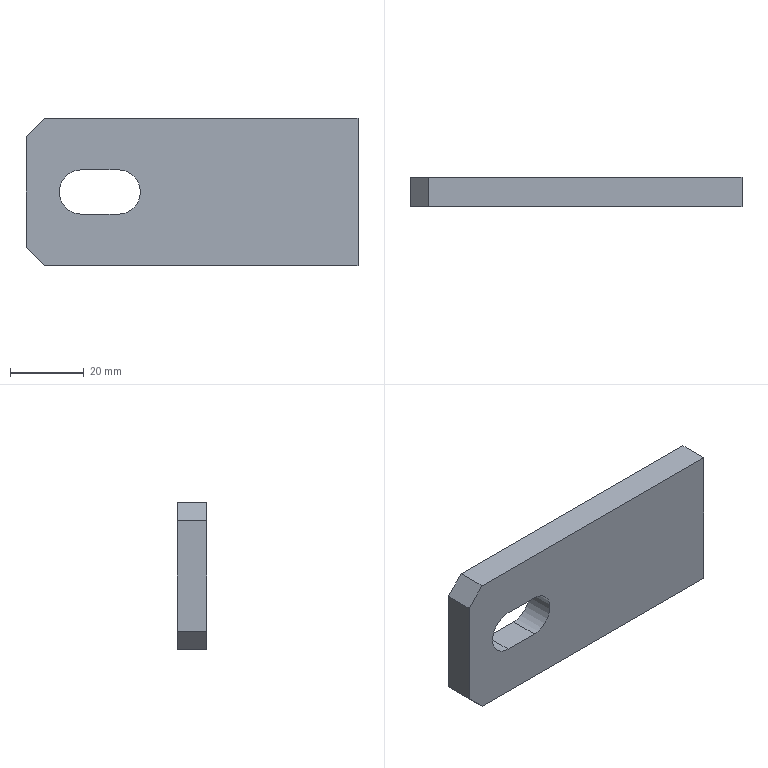Part | STEP file | E3-Guardrail base plate 1 | 1 solid | 12 faces | box 90 x 8 x 40 mm | volume 26735 mm3 | plane 10 | cylinder 2 | commonest cylinder face diameters 12 x2
STEP:
#1=CARTESIAN_POINT('',(0.,0.,0.));
#2=DIRECTION('',(0.,0.,1.));
#3=DIRECTION('',(1.,0.,0.));
#4=AXIS2_PLACEMENT_3D('',#1,#2,#3);
#5=CARTESIAN_POINT('',(45.,0.,-20.));
#6=VERTEX_POINT('',#5);
#7=CARTESIAN_POINT('',(45.,0.,20.));
#8=VERTEX_POINT('',#7);
#9=CARTESIAN_POINT('',(45.,0.,20.));
#10=DIRECTION('',(0.,0.,1.));
#11=VECTOR('',#10,1.);
#12=LINE('',#9,#11);
#13=CARTESIAN_POINT('',(45.,8.,20.));
#14=DIRECTION('',(-1.,0.,0.));
#15=DIRECTION('',(0.,0.,-1.));
#16=AXIS2_PLACEMENT_3D('',#13,#14,#15);
#17=PLANE('',#16);
#18=CARTESIAN_POINT('',(0.,8.));
#19=DIRECTION('',(-1.,0.));
#20=VECTOR('',#19,1.);
#21=LINE('',#18,#20);
#22=(GEOMETRIC_REPRESENTATION_CONTEXT(2)PARAMETRIC_REPRESENTATION_CONTEXT()REPRESENTATION_CONTEXT('',''));
#23=DEFINITIONAL_REPRESENTATION('',(#21),#22);
#24=PCURVE('',#17,#23);
#25=CARTESIAN_POINT('',(0.,0.,0.));
#26=DIRECTION('',(0.,1.,0.));
#27=DIRECTION('',(0.,0.,-1.));
#28=AXIS2_PLACEMENT_3D('',#25,#26,#27);
#29=PLANE('',#28);
#30=CARTESIAN_POINT('',(-20.,-45.));
#31=DIRECTION('',(-1.,0.));
#32=VECTOR('',#31,1.);
#33=LINE('',#30,#32);
#34=(GEOMETRIC_REPRESENTATION_CONTEXT(2)PARAMETRIC_REPRESENTATION_CONTEXT()REPRESENTATION_CONTEXT('',''));
#35=DEFINITIONAL_REPRESENTATION('',(#33),#34);
#36=PCURVE('',#29,#35);
#37=SURFACE_CURVE('',#12,(#24,#36),.PCURVE_S1.);
#38=EDGE_CURVE('',#6,#8,#37,.T.);
#39=ORIENTED_EDGE('',*,*,#38,.F.);
#40=CARTESIAN_POINT('',(45.,8.,-20.));
#41=VERTEX_POINT('',#40);
#42=CARTESIAN_POINT('',(45.,8.,-20.));
#43=DIRECTION('',(0.,-1.,0.));
#44=VECTOR('',#43,1.);
#45=LINE('',#42,#44);
#46=CARTESIAN_POINT('',(40.,0.));
#47=DIRECTION('',(0.,1.));
#48=VECTOR('',#47,1.);
#49=LINE('',#46,#48);
#50=(GEOMETRIC_REPRESENTATION_CONTEXT(2)PARAMETRIC_REPRESENTATION_CONTEXT()REPRESENTATION_CONTEXT('',''));
#51=DEFINITIONAL_REPRESENTATION('',(#49),#50);
#52=PCURVE('',#17,#51);
#53=CARTESIAN_POINT('',(-45.,8.,-20.));
#54=DIRECTION('',(0.,0.,1.));
#55=DIRECTION('',(-1.,0.,0.));
#56=AXIS2_PLACEMENT_3D('',#53,#54,#55);
#57=PLANE('',#56);
#58=CARTESIAN_POINT('',(-90.,0.));
#59=DIRECTION('',(0.,1.));
#60=VECTOR('',#59,1.);
#61=LINE('',#58,#60);
#62=(GEOMETRIC_REPRESENTATION_CONTEXT(2)PARAMETRIC_REPRESENTATION_CONTEXT()REPRESENTATION_CONTEXT('',''));
#63=DEFINITIONAL_REPRESENTATION('',(#61),#62);
#64=PCURVE('',#57,#63);
#65=SURFACE_CURVE('',#45,(#52,#64),.PCURVE_S1.);
#66=EDGE_CURVE('',#41,#6,#65,.T.);
#67=ORIENTED_EDGE('',*,*,#66,.F.);
#68=CARTESIAN_POINT('',(45.,8.,20.));
#69=VERTEX_POINT('',#68);
#70=CARTESIAN_POINT('',(45.,8.,20.));
#71=DIRECTION('',(0.,0.,1.));
#72=VECTOR('',#71,1.);
#73=LINE('',#70,#72);
#74=CARTESIAN_POINT('',(0.,0.));
#75=DIRECTION('',(-1.,0.));
#76=VECTOR('',#75,1.);
#77=LINE('',#74,#76);
#78=(GEOMETRIC_REPRESENTATION_CONTEXT(2)PARAMETRIC_REPRESENTATION_CONTEXT()REPRESENTATION_CONTEXT('',''));
#79=DEFINITIONAL_REPRESENTATION('',(#77),#78);
#80=PCURVE('',#17,#79);
#81=CARTESIAN_POINT('',(0.,8.,0.));
#82=DIRECTION('',(0.,1.,0.));
#83=DIRECTION('',(0.,0.,-1.));
#84=AXIS2_PLACEMENT_3D('',#81,#82,#83);
#85=PLANE('',#84);
#86=CARTESIAN_POINT('',(-20.,-45.));
#87=DIRECTION('',(-1.,0.));
#88=VECTOR('',#87,1.);
#89=LINE('',#86,#88);
#90=(GEOMETRIC_REPRESENTATION_CONTEXT(2)PARAMETRIC_REPRESENTATION_CONTEXT()REPRESENTATION_CONTEXT('',''));
#91=DEFINITIONAL_REPRESENTATION('',(#89),#90);
#92=PCURVE('',#85,#91);
#93=SURFACE_CURVE('',#73,(#80,#92),.PCURVE_S1.);
#94=EDGE_CURVE('',#41,#69,#93,.T.);
#95=ORIENTED_EDGE('',*,*,#94,.T.);
#96=CARTESIAN_POINT('',(45.,8.,20.));
#97=DIRECTION('',(0.,-1.,0.));
#98=VECTOR('',#97,1.);
#99=LINE('',#96,#98);
#100=CARTESIAN_POINT('',(0.,0.));
#101=DIRECTION('',(0.,1.));
#102=VECTOR('',#101,1.);
#103=LINE('',#100,#102);
#104=(GEOMETRIC_REPRESENTATION_CONTEXT(2)PARAMETRIC_REPRESENTATION_CONTEXT()REPRESENTATION_CONTEXT('',''));
#105=DEFINITIONAL_REPRESENTATION('',(#103),#104);
#106=PCURVE('',#17,#105);
#107=CARTESIAN_POINT('',(-45.,8.,20.));
#108=DIRECTION('',(0.,0.,-1.));
#109=DIRECTION('',(1.,0.,0.));
#110=AXIS2_PLACEMENT_3D('',#107,#108,#109);
#111=PLANE('',#110);
#112=CARTESIAN_POINT('',(90.,0.));
#113=DIRECTION('',(0.,1.));
#114=VECTOR('',#113,1.);
#115=LINE('',#112,#114);
#116=(GEOMETRIC_REPRESENTATION_CONTEXT(2)PARAMETRIC_REPRESENTATION_CONTEXT()REPRESENTATION_CONTEXT('',''));
#117=DEFINITIONAL_REPRESENTATION('',(#115),#116);
#118=PCURVE('',#111,#117);
#119=SURFACE_CURVE('',#99,(#106,#118),.PCURVE_S1.);
#120=EDGE_CURVE('',#69,#8,#119,.T.);
#121=ORIENTED_EDGE('',*,*,#120,.T.);
#122=EDGE_LOOP('',(#39,#67,#95,#121));
#123=FACE_BOUND('',#122,.T.);
#124=ADVANCED_FACE('',(#123),#17,.F.);
#125=CARTESIAN_POINT('',(-40.,0.,20.));
#126=VERTEX_POINT('',#125);
#127=CARTESIAN_POINT('',(-45.,0.,20.));
#128=DIRECTION('',(-1.,0.,0.));
#129=VECTOR('',#128,1.);
#130=LINE('',#127,#129);
#131=CARTESIAN_POINT('',(0.,8.));
#132=DIRECTION('',(-1.,0.));
#133=VECTOR('',#132,1.);
#134=LINE('',#131,#133);
#135=(GEOMETRIC_REPRESENTATION_CONTEXT(2)PARAMETRIC_REPRESENTATION_CONTEXT()REPRESENTATION_CONTEXT('',''));
#136=DEFINITIONAL_REPRESENTATION('',(#134),#135);
#137=PCURVE('',#111,#136);
#138=CARTESIAN_POINT('',(-20.,45.));
#139=DIRECTION('',(0.,1.));
#140=VECTOR('',#139,1.);
#141=LINE('',#138,#140);
#142=(GEOMETRIC_REPRESENTATION_CONTEXT(2)PARAMETRIC_REPRESENTATION_CONTEXT()REPRESENTATION_CONTEXT('',''));
#143=DEFINITIONAL_REPRESENTATION('',(#141),#142);
#144=PCURVE('',#29,#143);
#145=SURFACE_CURVE('',#130,(#137,#144),.PCURVE_S1.);
#146=EDGE_CURVE('',#8,#126,#145,.T.);
#147=ORIENTED_EDGE('',*,*,#146,.F.);
#148=ORIENTED_EDGE('',*,*,#120,.F.);
#149=CARTESIAN_POINT('',(-40.,8.,20.));
#150=VERTEX_POINT('',#149);
#151=CARTESIAN_POINT('',(-45.,8.,20.));
#152=DIRECTION('',(-1.,0.,0.));
#153=VECTOR('',#152,1.);
#154=LINE('',#151,#153);
#155=CARTESIAN_POINT('',(0.,0.));
#156=DIRECTION('',(-1.,0.));
#157=VECTOR('',#156,1.);
#158=LINE('',#155,#157);
#159=(GEOMETRIC_REPRESENTATION_CONTEXT(2)PARAMETRIC_REPRESENTATION_CONTEXT()REPRESENTATION_CONTEXT('',''));
#160=DEFINITIONAL_REPRESENTATION('',(#158),#159);
#161=PCURVE('',#111,#160);
#162=CARTESIAN_POINT('',(-20.,45.));
#163=DIRECTION('',(0.,1.));
#164=VECTOR('',#163,1.);
#165=LINE('',#162,#164);
#166=(GEOMETRIC_REPRESENTATION_CONTEXT(2)PARAMETRIC_REPRESENTATION_CONTEXT()REPRESENTATION_CONTEXT('',''));
#167=DEFINITIONAL_REPRESENTATION('',(#165),#166);
#168=PCURVE('',#85,#167);
#169=SURFACE_CURVE('',#154,(#161,#168),.PCURVE_S1.);
#170=EDGE_CURVE('',#69,#150,#169,.T.);
#171=ORIENTED_EDGE('',*,*,#170,.T.);
#172=CARTESIAN_POINT('',(-40.,8.,20.));
#173=DIRECTION('',(0.,1.,0.));
#174=VECTOR('',#173,1.);
#175=LINE('',#172,#174);
#176=CARTESIAN_POINT('',(5.,0.));
#177=DIRECTION('',(0.,-1.));
#178=VECTOR('',#177,1.);
#179=LINE('',#176,#178);
#180=(GEOMETRIC_REPRESENTATION_CONTEXT(2)PARAMETRIC_REPRESENTATION_CONTEXT()REPRESENTATION_CONTEXT('',''));
#181=DEFINITIONAL_REPRESENTATION('',(#179),#180);
#182=PCURVE('',#111,#181);
#183=CARTESIAN_POINT('',(-45.,8.,15.));
#184=DIRECTION('',(0.7071,0.,-0.7071));
#185=DIRECTION('',(0.,-1.,0.));
#186=AXIS2_PLACEMENT_3D('',#183,#184,#185);
#187=PLANE('',#186);
#188=CARTESIAN_POINT('',(0.,-7.071));
#189=DIRECTION('',(-1.,0.));
#190=VECTOR('',#189,1.);
#191=LINE('',#188,#190);
#192=(GEOMETRIC_REPRESENTATION_CONTEXT(2)PARAMETRIC_REPRESENTATION_CONTEXT()REPRESENTATION_CONTEXT('',''));
#193=DEFINITIONAL_REPRESENTATION('',(#191),#192);
#194=PCURVE('',#187,#193);
#195=SURFACE_CURVE('',#175,(#182,#194),.PCURVE_S1.);
#196=EDGE_CURVE('',#126,#150,#195,.T.);
#197=ORIENTED_EDGE('',*,*,#196,.F.);
#198=EDGE_LOOP('',(#147,#148,#171,#197));
#199=FACE_BOUND('',#198,.T.);
#200=ADVANCED_FACE('',(#199),#111,.F.);
#201=CARTESIAN_POINT('',(-45.,0.,15.));
#202=VERTEX_POINT('',#201);
#203=CARTESIAN_POINT('',(-45.,0.,-15.));
#204=VERTEX_POINT('',#203);
#205=CARTESIAN_POINT('',(-45.,0.,20.));
#206=DIRECTION('',(0.,0.,-1.));
#207=VECTOR('',#206,1.);
#208=LINE('',#205,#207);
#209=CARTESIAN_POINT('',(-45.,8.,20.));
#210=DIRECTION('',(1.,0.,0.));
#211=DIRECTION('',(0.,0.,1.));
#212=AXIS2_PLACEMENT_3D('',#209,#210,#211);
#213=PLANE('',#212);
#214=CARTESIAN_POINT('',(0.,8.));
#215=DIRECTION('',(-1.,0.));
#216=VECTOR('',#215,1.);
#217=LINE('',#214,#216);
#218=(GEOMETRIC_REPRESENTATION_CONTEXT(2)PARAMETRIC_REPRESENTATION_CONTEXT()REPRESENTATION_CONTEXT('',''));
#219=DEFINITIONAL_REPRESENTATION('',(#217),#218);
#220=PCURVE('',#213,#219);
#221=CARTESIAN_POINT('',(-20.,45.));
#222=DIRECTION('',(1.,0.));
#223=VECTOR('',#222,1.);
#224=LINE('',#221,#223);
#225=(GEOMETRIC_REPRESENTATION_CONTEXT(2)PARAMETRIC_REPRESENTATION_CONTEXT()REPRESENTATION_CONTEXT('',''));
#226=DEFINITIONAL_REPRESENTATION('',(#224),#225);
#227=PCURVE('',#29,#226);
#228=SURFACE_CURVE('',#208,(#220,#227),.PCURVE_S1.);
#229=EDGE_CURVE('',#202,#204,#228,.T.);
#230=ORIENTED_EDGE('',*,*,#229,.F.);
#231=CARTESIAN_POINT('',(-45.,8.,15.));
#232=VERTEX_POINT('',#231);
#233=CARTESIAN_POINT('',(-45.,8.,15.));
#234=DIRECTION('',(0.,-1.,0.));
#235=VECTOR('',#234,1.);
#236=LINE('',#233,#235);
#237=CARTESIAN_POINT('',(-5.,0.));
#238=DIRECTION('',(0.,1.));
#239=VECTOR('',#238,1.);
#240=LINE('',#237,#239);
#241=(GEOMETRIC_REPRESENTATION_CONTEXT(2)PARAMETRIC_REPRESENTATION_CONTEXT()REPRESENTATION_CONTEXT('',''));
#242=DEFINITIONAL_REPRESENTATION('',(#240),#241);
#243=PCURVE('',#213,#242);
#244=CARTESIAN_POINT('',(0.,0.));
#245=DIRECTION('',(1.,0.));
#246=VECTOR('',#245,1.);
#247=LINE('',#244,#246);
#248=(GEOMETRIC_REPRESENTATION_CONTEXT(2)PARAMETRIC_REPRESENTATION_CONTEXT()REPRESENTATION_CONTEXT('',''));
#249=DEFINITIONAL_REPRESENTATION('',(#247),#248);
#250=PCURVE('',#187,#249);
#251=SURFACE_CURVE('',#236,(#243,#250),.PCURVE_S1.);
#252=EDGE_CURVE('',#232,#202,#251,.T.);
#253=ORIENTED_EDGE('',*,*,#252,.F.);
#254=CARTESIAN_POINT('',(-45.,8.,-15.));
#255=VERTEX_POINT('',#254);
#256=CARTESIAN_POINT('',(-45.,8.,20.));
#257=DIRECTION('',(0.,0.,-1.));
#258=VECTOR('',#257,1.);
#259=LINE('',#256,#258);
#260=CARTESIAN_POINT('',(0.,0.));
#261=DIRECTION('',(-1.,0.));
#262=VECTOR('',#261,1.);
#263=LINE('',#260,#262);
#264=(GEOMETRIC_REPRESENTATION_CONTEXT(2)PARAMETRIC_REPRESENTATION_CONTEXT()REPRESENTATION_CONTEXT('',''));
#265=DEFINITIONAL_REPRESENTATION('',(#263),#264);
#266=PCURVE('',#213,#265);
#267=CARTESIAN_POINT('',(-20.,45.));
#268=DIRECTION('',(1.,0.));
#269=VECTOR('',#268,1.);
#270=LINE('',#267,#269);
#271=(GEOMETRIC_REPRESENTATION_CONTEXT(2)PARAMETRIC_REPRESENTATION_CONTEXT()REPRESENTATION_CONTEXT('',''));
#272=DEFINITIONAL_REPRESENTATION('',(#270),#271);
#273=PCURVE('',#85,#272);
#274=SURFACE_CURVE('',#259,(#266,#273),.PCURVE_S1.);
#275=EDGE_CURVE('',#232,#255,#274,.T.);
#276=ORIENTED_EDGE('',*,*,#275,.T.);
#277=CARTESIAN_POINT('',(-45.,8.,-15.));
#278=DIRECTION('',(0.,1.,0.));
#279=VECTOR('',#278,1.);
#280=LINE('',#277,#279);
#281=CARTESIAN_POINT('',(-35.,0.));
#282=DIRECTION('',(0.,-1.));
#283=VECTOR('',#282,1.);
#284=LINE('',#281,#283);
#285=(GEOMETRIC_REPRESENTATION_CONTEXT(2)PARAMETRIC_REPRESENTATION_CONTEXT()REPRESENTATION_CONTEXT('',''));
#286=DEFINITIONAL_REPRESENTATION('',(#284),#285);
#287=PCURVE('',#213,#286);
#288=CARTESIAN_POINT('',(-40.,8.,-20.));
#289=DIRECTION('',(0.7071,0.,0.7071));
#290=DIRECTION('',(0.,-1.,0.));
#291=AXIS2_PLACEMENT_3D('',#288,#289,#290);
#292=PLANE('',#291);
#293=CARTESIAN_POINT('',(0.,-7.071));
#294=DIRECTION('',(-1.,0.));
#295=VECTOR('',#294,1.);
#296=LINE('',#293,#295);
#297=(GEOMETRIC_REPRESENTATION_CONTEXT(2)PARAMETRIC_REPRESENTATION_CONTEXT()REPRESENTATION_CONTEXT('',''));
#298=DEFINITIONAL_REPRESENTATION('',(#296),#297);
#299=PCURVE('',#292,#298);
#300=SURFACE_CURVE('',#280,(#287,#299),.PCURVE_S1.);
#301=EDGE_CURVE('',#204,#255,#300,.T.);
#302=ORIENTED_EDGE('',*,*,#301,.F.);
#303=EDGE_LOOP('',(#230,#253,#276,#302));
#304=FACE_BOUND('',#303,.T.);
#305=ADVANCED_FACE('',(#304),#213,.F.);
#306=CARTESIAN_POINT('',(-40.,8.,-20.));
#307=VERTEX_POINT('',#306);
#308=CARTESIAN_POINT('',(-45.,8.,-20.));
#309=DIRECTION('',(1.,0.,0.));
#310=VECTOR('',#309,1.);
#311=LINE('',#308,#310);
#312=CARTESIAN_POINT('',(0.,0.));
#313=DIRECTION('',(-1.,0.));
#314=VECTOR('',#313,1.);
#315=LINE('',#312,#314);
#316=(GEOMETRIC_REPRESENTATION_CONTEXT(2)PARAMETRIC_REPRESENTATION_CONTEXT()REPRESENTATION_CONTEXT('',''));
#317=DEFINITIONAL_REPRESENTATION('',(#315),#316);
#318=PCURVE('',#57,#317);
#319=CARTESIAN_POINT('',(20.,45.));
#320=DIRECTION('',(0.,-1.));
#321=VECTOR('',#320,1.);
#322=LINE('',#319,#321);
#323=(GEOMETRIC_REPRESENTATION_CONTEXT(2)PARAMETRIC_REPRESENTATION_CONTEXT()REPRESENTATION_CONTEXT('',''));
#324=DEFINITIONAL_REPRESENTATION('',(#322),#323);
#325=PCURVE('',#85,#324);
#326=SURFACE_CURVE('',#311,(#318,#325),.PCURVE_S1.);
#327=EDGE_CURVE('',#307,#41,#326,.T.);
#328=ORIENTED_EDGE('',*,*,#327,.T.);
#329=ORIENTED_EDGE('',*,*,#66,.T.);
#330=CARTESIAN_POINT('',(-40.,0.,-20.));
#331=VERTEX_POINT('',#330);
#332=CARTESIAN_POINT('',(-45.,0.,-20.));
#333=DIRECTION('',(1.,0.,0.));
#334=VECTOR('',#333,1.);
#335=LINE('',#332,#334);
#336=CARTESIAN_POINT('',(0.,8.));
#337=DIRECTION('',(-1.,0.));
#338=VECTOR('',#337,1.);
#339=LINE('',#336,#338);
#340=(GEOMETRIC_REPRESENTATION_CONTEXT(2)PARAMETRIC_REPRESENTATION_CONTEXT()REPRESENTATION_CONTEXT('',''));
#341=DEFINITIONAL_REPRESENTATION('',(#339),#340);
#342=PCURVE('',#57,#341);
#343=CARTESIAN_POINT('',(20.,45.));
#344=DIRECTION('',(0.,-1.));
#345=VECTOR('',#344,1.);
#346=LINE('',#343,#345);
#347=(GEOMETRIC_REPRESENTATION_CONTEXT(2)PARAMETRIC_REPRESENTATION_CONTEXT()REPRESENTATION_CONTEXT('',''));
#348=DEFINITIONAL_REPRESENTATION('',(#346),#347);
#349=PCURVE('',#29,#348);
#350=SURFACE_CURVE('',#335,(#342,#349),.PCURVE_S1.);
#351=EDGE_CURVE('',#331,#6,#350,.T.);
#352=ORIENTED_EDGE('',*,*,#351,.F.);
#353=CARTESIAN_POINT('',(-40.,8.,-20.));
#354=DIRECTION('',(0.,-1.,0.));
#355=VECTOR('',#354,1.);
#356=LINE('',#353,#355);
#357=CARTESIAN_POINT('',(-5.,0.));
#358=DIRECTION('',(0.,1.));
#359=VECTOR('',#358,1.);
#360=LINE('',#357,#359);
#361=(GEOMETRIC_REPRESENTATION_CONTEXT(2)PARAMETRIC_REPRESENTATION_CONTEXT()REPRESENTATION_CONTEXT('',''));
#362=DEFINITIONAL_REPRESENTATION('',(#360),#361);
#363=PCURVE('',#57,#362);
#364=CARTESIAN_POINT('',(0.,0.));
#365=DIRECTION('',(1.,0.));
#366=VECTOR('',#365,1.);
#367=LINE('',#364,#366);
#368=(GEOMETRIC_REPRESENTATION_CONTEXT(2)PARAMETRIC_REPRESENTATION_CONTEXT()REPRESENTATION_CONTEXT('',''));
#369=DEFINITIONAL_REPRESENTATION('',(#367),#368);
#370=PCURVE('',#292,#369);
#371=SURFACE_CURVE('',#356,(#363,#370),.PCURVE_S1.);
#372=EDGE_CURVE('',#307,#331,#371,.T.);
#373=ORIENTED_EDGE('',*,*,#372,.F.);
#374=EDGE_LOOP('',(#328,#329,#352,#373));
#375=FACE_BOUND('',#374,.T.);
#376=ADVANCED_FACE('',(#375),#57,.F.);
#377=CARTESIAN_POINT('',(-20.,8.,-6.));
#378=VERTEX_POINT('',#377);
#379=CARTESIAN_POINT('',(-20.,8.,6.));
#380=VERTEX_POINT('',#379);
#381=CARTESIAN_POINT('',(-20.,8.,0.));
#382=DIRECTION('',(0.,-1.,0.));
#383=DIRECTION('',(0.,0.,-1.));
#384=AXIS2_PLACEMENT_3D('',#381,#382,#383);
#385=CIRCLE('',#384,6.);
#386=CARTESIAN_POINT('',(6.,20.));
#387=CARTESIAN_POINT('',(6.,9.608));
#388=CARTESIAN_POINT('',(-3.,14.804));
#389=CARTESIAN_POINT('',(-12.,20.));
#390=CARTESIAN_POINT('',(-3.,25.196));
#391=CARTESIAN_POINT('',(6.,30.392));
#392=CARTESIAN_POINT('',(6.,20.));
#393=(BOUNDED_CURVE()B_SPLINE_CURVE(2,(#386,#387,#388,#389,#390,#391,#392),.UNSPECIFIED.,.T.,.F.)B_SPLINE_CURVE_WITH_KNOTS((1,2,2,2,2,1),(-2.094,0.,2.094,4.189,6.283,8.378),.UNSPECIFIED.)CURVE()GEOMETRIC_REPRESENTATION_ITEM()RATIONAL_B_SPLINE_CURVE((1.,0.5,1.,0.5,1.,0.5,1.))REPRESENTATION_ITEM(''));
#394=(GEOMETRIC_REPRESENTATION_CONTEXT(2)PARAMETRIC_REPRESENTATION_CONTEXT()REPRESENTATION_CONTEXT('',''));
#395=DEFINITIONAL_REPRESENTATION('',(#393),#394);
#396=PCURVE('',#85,#395);
#397=CARTESIAN_POINT('',(-20.,8.,0.));
#398=DIRECTION('',(0.,1.,0.));
#399=DIRECTION('',(0.,0.,-1.));
#400=AXIS2_PLACEMENT_3D('',#397,#398,#399);
#401=CYLINDRICAL_SURFACE('',#400,6.);
#402=CARTESIAN_POINT('',(6.283,0.));
#403=DIRECTION('',(-1.,0.));
#404=VECTOR('',#403,1.);
#405=LINE('',#402,#404);
#406=(GEOMETRIC_REPRESENTATION_CONTEXT(2)PARAMETRIC_REPRESENTATION_CONTEXT()REPRESENTATION_CONTEXT('',''));
#407=DEFINITIONAL_REPRESENTATION('',(#405),#406);
#408=PCURVE('',#401,#407);
#409=SURFACE_CURVE('',#385,(#396,#408),.PCURVE_S1.);
#410=EDGE_CURVE('',#378,#380,#409,.T.);
#411=ORIENTED_EDGE('',*,*,#410,.T.);
#412=CARTESIAN_POINT('',(-30.,8.,6.));
#413=VERTEX_POINT('',#412);
#414=CARTESIAN_POINT('',(-30.,8.,6.));
#415=DIRECTION('',(1.,0.,0.));
#416=VECTOR('',#415,1.);
#417=LINE('',#414,#416);
#418=CARTESIAN_POINT('',(-6.,30.));
#419=DIRECTION('',(0.,-1.));
#420=VECTOR('',#419,1.);
#421=LINE('',#418,#420);
#422=(GEOMETRIC_REPRESENTATION_CONTEXT(2)PARAMETRIC_REPRESENTATION_CONTEXT()REPRESENTATION_CONTEXT('',''));
#423=DEFINITIONAL_REPRESENTATION('',(#421),#422);
#424=PCURVE('',#85,#423);
#425=CARTESIAN_POINT('',(-30.,8.,6.));
#426=DIRECTION('',(0.,0.,1.));
#427=DIRECTION('',(-1.,0.,0.));
#428=AXIS2_PLACEMENT_3D('',#425,#426,#427);
#429=PLANE('',#428);
#430=CARTESIAN_POINT('',(0.,0.));
#431=DIRECTION('',(-1.,0.));
#432=VECTOR('',#431,1.);
#433=LINE('',#430,#432);
#434=(GEOMETRIC_REPRESENTATION_CONTEXT(2)PARAMETRIC_REPRESENTATION_CONTEXT()REPRESENTATION_CONTEXT('',''));
#435=DEFINITIONAL_REPRESENTATION('',(#433),#434);
#436=PCURVE('',#429,#435);
#437=SURFACE_CURVE('',#417,(#424,#436),.PCURVE_S1.);
#438=EDGE_CURVE('',#413,#380,#437,.T.);
#439=ORIENTED_EDGE('',*,*,#438,.F.);
#440=CARTESIAN_POINT('',(-30.,8.,-6.));
#441=VERTEX_POINT('',#440);
#442=CARTESIAN_POINT('',(-30.,8.,0.));
#443=DIRECTION('',(0.,-1.,0.));
#444=DIRECTION('',(0.,0.,-1.));
#445=AXIS2_PLACEMENT_3D('',#442,#443,#444);
#446=CIRCLE('',#445,6.);
#447=CARTESIAN_POINT('',(6.,30.));
#448=CARTESIAN_POINT('',(6.,19.608));
#449=CARTESIAN_POINT('',(-3.,24.804));
#450=CARTESIAN_POINT('',(-12.,30.));
#451=CARTESIAN_POINT('',(-3.,35.196));
#452=CARTESIAN_POINT('',(6.,40.392));
#453=CARTESIAN_POINT('',(6.,30.));
#454=(BOUNDED_CURVE()B_SPLINE_CURVE(2,(#447,#448,#449,#450,#451,#452,#453),.UNSPECIFIED.,.T.,.F.)B_SPLINE_CURVE_WITH_KNOTS((1,2,2,2,2,1),(-2.094,0.,2.094,4.189,6.283,8.378),.UNSPECIFIED.)CURVE()GEOMETRIC_REPRESENTATION_ITEM()RATIONAL_B_SPLINE_CURVE((1.,0.5,1.,0.5,1.,0.5,1.))REPRESENTATION_ITEM(''));
#455=(GEOMETRIC_REPRESENTATION_CONTEXT(2)PARAMETRIC_REPRESENTATION_CONTEXT()REPRESENTATION_CONTEXT('',''));
#456=DEFINITIONAL_REPRESENTATION('',(#454),#455);
#457=PCURVE('',#85,#456);
#458=CARTESIAN_POINT('',(-30.,8.,0.));
#459=DIRECTION('',(0.,1.,0.));
#460=DIRECTION('',(0.,0.,-1.));
#461=AXIS2_PLACEMENT_3D('',#458,#459,#460);
#462=CYLINDRICAL_SURFACE('',#461,6.);
#463=CARTESIAN_POINT('',(6.283,0.));
#464=DIRECTION('',(-1.,0.));
#465=VECTOR('',#464,1.);
#466=LINE('',#463,#465);
#467=(GEOMETRIC_REPRESENTATION_CONTEXT(2)PARAMETRIC_REPRESENTATION_CONTEXT()REPRESENTATION_CONTEXT('',''));
#468=DEFINITIONAL_REPRESENTATION('',(#466),#467);
#469=PCURVE('',#462,#468);
#470=SURFACE_CURVE('',#446,(#457,#469),.PCURVE_S1.);
#471=EDGE_CURVE('',#413,#441,#470,.T.);
#472=ORIENTED_EDGE('',*,*,#471,.T.);
#473=CARTESIAN_POINT('',(-30.,8.,-6.));
#474=DIRECTION('',(1.,0.,0.));
#475=VECTOR('',#474,1.);
#476=LINE('',#473,#475);
#477=CARTESIAN_POINT('',(6.,30.));
#478=DIRECTION('',(0.,-1.));
#479=VECTOR('',#478,1.);
#480=LINE('',#477,#479);
#481=(GEOMETRIC_REPRESENTATION_CONTEXT(2)PARAMETRIC_REPRESENTATION_CONTEXT()REPRESENTATION_CONTEXT('',''));
#482=DEFINITIONAL_REPRESENTATION('',(#480),#481);
#483=PCURVE('',#85,#482);
#484=CARTESIAN_POINT('',(-30.,8.,-6.));
#485=DIRECTION('',(0.,0.,-1.));
#486=DIRECTION('',(1.,0.,0.));
#487=AXIS2_PLACEMENT_3D('',#484,#485,#486);
#488=PLANE('',#487);
#489=CARTESIAN_POINT('',(0.,0.));
#490=DIRECTION('',(1.,0.));
#491=VECTOR('',#490,1.);
#492=LINE('',#489,#491);
#493=(GEOMETRIC_REPRESENTATION_CONTEXT(2)PARAMETRIC_REPRESENTATION_CONTEXT()REPRESENTATION_CONTEXT('',''));
#494=DEFINITIONAL_REPRESENTATION('',(#492),#493);
#495=PCURVE('',#488,#494);
#496=SURFACE_CURVE('',#476,(#483,#495),.PCURVE_S1.);
#497=EDGE_CURVE('',#441,#378,#496,.T.);
#498=ORIENTED_EDGE('',*,*,#497,.T.);
#499=EDGE_LOOP('',(#411,#439,#472,#498));
#500=FACE_BOUND('',#499,.T.);
#501=ORIENTED_EDGE('',*,*,#275,.F.);
#502=CARTESIAN_POINT('',(-30.,8.,30.));
#503=DIRECTION('',(-0.7071,0.,-0.7071));
#504=VECTOR('',#503,1.);
#505=LINE('',#502,#504);
#506=CARTESIAN_POINT('',(-30.,30.));
#507=DIRECTION('',(0.7071,0.7071));
#508=VECTOR('',#507,1.);
#509=LINE('',#506,#508);
#510=(GEOMETRIC_REPRESENTATION_CONTEXT(2)PARAMETRIC_REPRESENTATION_CONTEXT()REPRESENTATION_CONTEXT('',''));
#511=DEFINITIONAL_REPRESENTATION('',(#509),#510);
#512=PCURVE('',#85,#511);
#513=CARTESIAN_POINT('',(0.,-21.213));
#514=DIRECTION('',(0.,1.));
#515=VECTOR('',#514,1.);
#516=LINE('',#513,#515);
#517=(GEOMETRIC_REPRESENTATION_CONTEXT(2)PARAMETRIC_REPRESENTATION_CONTEXT()REPRESENTATION_CONTEXT('',''));
#518=DEFINITIONAL_REPRESENTATION('',(#516),#517);
#519=PCURVE('',#187,#518);
#520=SURFACE_CURVE('',#505,(#512,#519),.PCURVE_S1.);
#521=EDGE_CURVE('',#150,#232,#520,.T.);
#522=ORIENTED_EDGE('',*,*,#521,.F.);
#523=ORIENTED_EDGE('',*,*,#170,.F.);
#524=ORIENTED_EDGE('',*,*,#94,.F.);
#525=ORIENTED_EDGE('',*,*,#327,.F.);
#526=CARTESIAN_POINT('',(-30.,8.,-30.));
#527=DIRECTION('',(0.7071,0.,-0.7071));
#528=VECTOR('',#527,1.);
#529=LINE('',#526,#528);
#530=CARTESIAN_POINT('',(30.,30.));
#531=DIRECTION('',(0.7071,-0.7071));
#532=VECTOR('',#531,1.);
#533=LINE('',#530,#532);
#534=(GEOMETRIC_REPRESENTATION_CONTEXT(2)PARAMETRIC_REPRESENTATION_CONTEXT()REPRESENTATION_CONTEXT('',''));
#535=DEFINITIONAL_REPRESENTATION('',(#533),#534);
#536=PCURVE('',#85,#535);
#537=CARTESIAN_POINT('',(0.,14.142));
#538=DIRECTION('',(0.,1.));
#539=VECTOR('',#538,1.);
#540=LINE('',#537,#539);
#541=(GEOMETRIC_REPRESENTATION_CONTEXT(2)PARAMETRIC_REPRESENTATION_CONTEXT()REPRESENTATION_CONTEXT('',''));
#542=DEFINITIONAL_REPRESENTATION('',(#540),#541);
#543=PCURVE('',#292,#542);
#544=SURFACE_CURVE('',#529,(#536,#543),.PCURVE_S1.);
#545=EDGE_CURVE('',#255,#307,#544,.T.);
#546=ORIENTED_EDGE('',*,*,#545,.F.);
#547=EDGE_LOOP('',(#501,#522,#523,#524,#525,#546));
#548=FACE_BOUND('',#547,.T.);
#549=ADVANCED_FACE('',(#500,#548),#85,.T.);
#550=CARTESIAN_POINT('',(-20.,0.,-6.));
#551=VERTEX_POINT('',#550);
#552=CARTESIAN_POINT('',(-20.,0.,6.));
#553=VERTEX_POINT('',#552);
#554=CARTESIAN_POINT('',(-20.,0.,0.));
#555=DIRECTION('',(0.,-1.,0.));
#556=DIRECTION('',(0.,0.,-1.));
#557=AXIS2_PLACEMENT_3D('',#554,#555,#556);
#558=CIRCLE('',#557,6.);
#559=CARTESIAN_POINT('',(6.,20.));
#560=CARTESIAN_POINT('',(6.,9.608));
#561=CARTESIAN_POINT('',(-3.,14.804));
#562=CARTESIAN_POINT('',(-12.,20.));
#563=CARTESIAN_POINT('',(-3.,25.196));
#564=CARTESIAN_POINT('',(6.,30.392));
#565=CARTESIAN_POINT('',(6.,20.));
#566=(BOUNDED_CURVE()B_SPLINE_CURVE(2,(#559,#560,#561,#562,#563,#564,#565),.UNSPECIFIED.,.T.,.F.)B_SPLINE_CURVE_WITH_KNOTS((1,2,2,2,2,1),(-2.094,0.,2.094,4.189,6.283,8.378),.UNSPECIFIED.)CURVE()GEOMETRIC_REPRESENTATION_ITEM()RATIONAL_B_SPLINE_CURVE((1.,0.5,1.,0.5,1.,0.5,1.))REPRESENTATION_ITEM(''));
#567=(GEOMETRIC_REPRESENTATION_CONTEXT(2)PARAMETRIC_REPRESENTATION_CONTEXT()REPRESENTATION_CONTEXT('',''));
#568=DEFINITIONAL_REPRESENTATION('',(#566),#567);
#569=PCURVE('',#29,#568);
#570=CARTESIAN_POINT('',(6.283,-8.));
#571=DIRECTION('',(-1.,0.));
#572=VECTOR('',#571,1.);
#573=LINE('',#570,#572);
#574=(GEOMETRIC_REPRESENTATION_CONTEXT(2)PARAMETRIC_REPRESENTATION_CONTEXT()REPRESENTATION_CONTEXT('',''));
#575=DEFINITIONAL_REPRESENTATION('',(#573),#574);
#576=PCURVE('',#401,#575);
#577=SURFACE_CURVE('',#558,(#569,#576),.PCURVE_S1.);
#578=EDGE_CURVE('',#551,#553,#577,.T.);
#579=ORIENTED_EDGE('',*,*,#578,.F.);
#580=CARTESIAN_POINT('',(-30.,0.,-6.));
#581=VERTEX_POINT('',#580);
#582=CARTESIAN_POINT('',(0.,0.,-6.));
#583=DIRECTION('',(1.,0.,0.));
#584=VECTOR('',#583,1.);
#585=LINE('',#582,#584);
#586=CARTESIAN_POINT('',(6.,0.));
#587=DIRECTION('',(0.,-1.));
#588=VECTOR('',#587,1.);
#589=LINE('',#586,#588);
#590=(GEOMETRIC_REPRESENTATION_CONTEXT(2)PARAMETRIC_REPRESENTATION_CONTEXT()REPRESENTATION_CONTEXT('',''));
#591=DEFINITIONAL_REPRESENTATION('',(#589),#590);
#592=PCURVE('',#29,#591);
#593=CARTESIAN_POINT('',(30.,8.));
#594=DIRECTION('',(1.,0.));
#595=VECTOR('',#594,1.);
#596=LINE('',#593,#595);
#597=(GEOMETRIC_REPRESENTATION_CONTEXT(2)PARAMETRIC_REPRESENTATION_CONTEXT()REPRESENTATION_CONTEXT('',''));
#598=DEFINITIONAL_REPRESENTATION('',(#596),#597);
#599=PCURVE('',#488,#598);
#600=SURFACE_CURVE('',#585,(#592,#599),.PCURVE_S1.);
#601=EDGE_CURVE('',#581,#551,#600,.T.);
#602=ORIENTED_EDGE('',*,*,#601,.F.);
#603=CARTESIAN_POINT('',(-30.,0.,6.));
#604=VERTEX_POINT('',#603);
#605=CARTESIAN_POINT('',(-30.,0.,0.));
#606=DIRECTION('',(0.,-1.,0.));
#607=DIRECTION('',(0.,0.,-1.));
#608=AXIS2_PLACEMENT_3D('',#605,#606,#607);
#609=CIRCLE('',#608,6.);
#610=CARTESIAN_POINT('',(6.,30.));
#611=CARTESIAN_POINT('',(6.,19.608));
#612=CARTESIAN_POINT('',(-3.,24.804));
#613=CARTESIAN_POINT('',(-12.,30.));
#614=CARTESIAN_POINT('',(-3.,35.196));
#615=CARTESIAN_POINT('',(6.,40.392));
#616=CARTESIAN_POINT('',(6.,30.));
#617=(BOUNDED_CURVE()B_SPLINE_CURVE(2,(#610,#611,#612,#613,#614,#615,#616),.UNSPECIFIED.,.T.,.F.)B_SPLINE_CURVE_WITH_KNOTS((1,2,2,2,2,1),(-2.094,0.,2.094,4.189,6.283,8.378),.UNSPECIFIED.)CURVE()GEOMETRIC_REPRESENTATION_ITEM()RATIONAL_B_SPLINE_CURVE((1.,0.5,1.,0.5,1.,0.5,1.))REPRESENTATION_ITEM(''));
#618=(GEOMETRIC_REPRESENTATION_CONTEXT(2)PARAMETRIC_REPRESENTATION_CONTEXT()REPRESENTATION_CONTEXT('',''));
#619=DEFINITIONAL_REPRESENTATION('',(#617),#618);
#620=PCURVE('',#29,#619);
#621=CARTESIAN_POINT('',(6.283,-8.));
#622=DIRECTION('',(-1.,0.));
#623=VECTOR('',#622,1.);
#624=LINE('',#621,#623);
#625=(GEOMETRIC_REPRESENTATION_CONTEXT(2)PARAMETRIC_REPRESENTATION_CONTEXT()REPRESENTATION_CONTEXT('',''));
#626=DEFINITIONAL_REPRESENTATION('',(#624),#625);
#627=PCURVE('',#462,#626);
#628=SURFACE_CURVE('',#609,(#620,#627),.PCURVE_S1.);
#629=EDGE_CURVE('',#604,#581,#628,.T.);
#630=ORIENTED_EDGE('',*,*,#629,.F.);
#631=CARTESIAN_POINT('',(0.,0.,6.));
#632=DIRECTION('',(-1.,0.,0.));
#633=VECTOR('',#632,1.);
#634=LINE('',#631,#633);
#635=CARTESIAN_POINT('',(-6.,0.));
#636=DIRECTION('',(0.,1.));
#637=VECTOR('',#636,1.);
#638=LINE('',#635,#637);
#639=(GEOMETRIC_REPRESENTATION_CONTEXT(2)PARAMETRIC_REPRESENTATION_CONTEXT()REPRESENTATION_CONTEXT('',''));
#640=DEFINITIONAL_REPRESENTATION('',(#638),#639);
#641=PCURVE('',#29,#640);
#642=CARTESIAN_POINT('',(-30.,8.));
#643=DIRECTION('',(1.,0.));
#644=VECTOR('',#643,1.);
#645=LINE('',#642,#644);
#646=(GEOMETRIC_REPRESENTATION_CONTEXT(2)PARAMETRIC_REPRESENTATION_CONTEXT()REPRESENTATION_CONTEXT('',''));
#647=DEFINITIONAL_REPRESENTATION('',(#645),#646);
#648=PCURVE('',#429,#647);
#649=SURFACE_CURVE('',#634,(#641,#648),.PCURVE_S1.);
#650=EDGE_CURVE('',#553,#604,#649,.T.);
#651=ORIENTED_EDGE('',*,*,#650,.F.);
#652=EDGE_LOOP('',(#579,#602,#630,#651));
#653=FACE_BOUND('',#652,.T.);
#654=ORIENTED_EDGE('',*,*,#351,.T.);
#655=ORIENTED_EDGE('',*,*,#38,.T.);
#656=ORIENTED_EDGE('',*,*,#146,.T.);
#657=CARTESIAN_POINT('',(-45.,0.,15.));
#658=DIRECTION('',(0.7071,0.,0.7071));
#659=VECTOR('',#658,1.);
#660=LINE('',#657,#659);
#661=CARTESIAN_POINT('',(-15.,45.));
#662=DIRECTION('',(-0.7071,-0.7071));
#663=VECTOR('',#662,1.);
#664=LINE('',#661,#663);
#665=(GEOMETRIC_REPRESENTATION_CONTEXT(2)PARAMETRIC_REPRESENTATION_CONTEXT()REPRESENTATION_CONTEXT('',''));
#666=DEFINITIONAL_REPRESENTATION('',(#664),#665);
#667=PCURVE('',#29,#666);
#668=CARTESIAN_POINT('',(8.,0.));
#669=DIRECTION('',(0.,-1.));
#670=VECTOR('',#669,1.);
#671=LINE('',#668,#670);
#672=(GEOMETRIC_REPRESENTATION_CONTEXT(2)PARAMETRIC_REPRESENTATION_CONTEXT()REPRESENTATION_CONTEXT('',''));
#673=DEFINITIONAL_REPRESENTATION('',(#671),#672);
#674=PCURVE('',#187,#673);
#675=SURFACE_CURVE('',#660,(#667,#674),.PCURVE_S1.);
#676=EDGE_CURVE('',#202,#126,#675,.T.);
#677=ORIENTED_EDGE('',*,*,#676,.F.);
#678=ORIENTED_EDGE('',*,*,#229,.T.);
#679=CARTESIAN_POINT('',(-40.,0.,-20.));
#680=DIRECTION('',(-0.7071,0.,0.7071));
#681=VECTOR('',#680,1.);
#682=LINE('',#679,#681);
#683=CARTESIAN_POINT('',(20.,40.));
#684=DIRECTION('',(-0.7071,0.7071));
#685=VECTOR('',#684,1.);
#686=LINE('',#683,#685);
#687=(GEOMETRIC_REPRESENTATION_CONTEXT(2)PARAMETRIC_REPRESENTATION_CONTEXT()REPRESENTATION_CONTEXT('',''));
#688=DEFINITIONAL_REPRESENTATION('',(#686),#687);
#689=PCURVE('',#29,#688);
#690=CARTESIAN_POINT('',(8.,0.));
#691=DIRECTION('',(0.,-1.));
#692=VECTOR('',#691,1.);
#693=LINE('',#690,#692);
#694=(GEOMETRIC_REPRESENTATION_CONTEXT(2)PARAMETRIC_REPRESENTATION_CONTEXT()REPRESENTATION_CONTEXT('',''));
#695=DEFINITIONAL_REPRESENTATION('',(#693),#694);
#696=PCURVE('',#292,#695);
#697=SURFACE_CURVE('',#682,(#689,#696),.PCURVE_S1.);
#698=EDGE_CURVE('',#331,#204,#697,.T.);
#699=ORIENTED_EDGE('',*,*,#698,.F.);
#700=EDGE_LOOP('',(#654,#655,#656,#677,#678,#699));
#701=FACE_BOUND('',#700,.T.);
#702=ADVANCED_FACE('',(#653,#701),#29,.F.);
#703=ORIENTED_EDGE('',*,*,#410,.T.);
#704=CARTESIAN_POINT('',(-20.,8.,6.));
#705=DIRECTION('',(0.,1.,0.));
#706=VECTOR('',#705,1.);
#707=LINE('',#704,#706);
#708=CARTESIAN_POINT('',(3.142,0.));
#709=DIRECTION('',(0.,1.));
#710=VECTOR('',#709,1.);
#711=LINE('',#708,#710);
#712=(GEOMETRIC_REPRESENTATION_CONTEXT(2)PARAMETRIC_REPRESENTATION_CONTEXT()REPRESENTATION_CONTEXT('',''));
#713=DEFINITIONAL_REPRESENTATION('',(#711),#712);
#714=PCURVE('',#401,#713);
#715=CARTESIAN_POINT('',(-10.,0.));
#716=DIRECTION('',(0.,-1.));
#717=VECTOR('',#716,1.);
#718=LINE('',#715,#717);
#719=(GEOMETRIC_REPRESENTATION_CONTEXT(2)PARAMETRIC_REPRESENTATION_CONTEXT()REPRESENTATION_CONTEXT('',''));
#720=DEFINITIONAL_REPRESENTATION('',(#718),#719);
#721=PCURVE('',#429,#720);
#722=SURFACE_CURVE('',#707,(#714,#721),.PCURVE_S1.);
#723=EDGE_CURVE('',#553,#380,#722,.T.);
#724=ORIENTED_EDGE('',*,*,#723,.F.);
#725=ORIENTED_EDGE('',*,*,#578,.F.);
#726=CARTESIAN_POINT('',(-20.,8.,-6.));
#727=DIRECTION('',(0.,-1.,0.));
#728=VECTOR('',#727,1.);
#729=LINE('',#726,#728);
#730=CARTESIAN_POINT('',(6.283,0.));
#731=DIRECTION('',(0.,-1.));
#732=VECTOR('',#731,1.);
#733=LINE('',#730,#732);
#734=(GEOMETRIC_REPRESENTATION_CONTEXT(2)PARAMETRIC_REPRESENTATION_CONTEXT()REPRESENTATION_CONTEXT('',''));
#735=DEFINITIONAL_REPRESENTATION('',(#733),#734);
#736=PCURVE('',#401,#735);
#737=CARTESIAN_POINT('',(10.,0.));
#738=DIRECTION('',(0.,1.));
#739=VECTOR('',#738,1.);
#740=LINE('',#737,#739);
#741=(GEOMETRIC_REPRESENTATION_CONTEXT(2)PARAMETRIC_REPRESENTATION_CONTEXT()REPRESENTATION_CONTEXT('',''));
#742=DEFINITIONAL_REPRESENTATION('',(#740),#741);
#743=PCURVE('',#488,#742);
#744=SURFACE_CURVE('',#729,(#736,#743),.PCURVE_S1.);
#745=EDGE_CURVE('',#378,#551,#744,.T.);
#746=ORIENTED_EDGE('',*,*,#745,.F.);
#747=EDGE_LOOP('',(#703,#724,#725,#746));
#748=FACE_BOUND('',#747,.F.);
#749=ADVANCED_FACE('',(#748),#401,.F.);
#750=ORIENTED_EDGE('',*,*,#471,.T.);
#751=CARTESIAN_POINT('',(-30.,8.,-6.));
#752=DIRECTION('',(0.,1.,0.));
#753=VECTOR('',#752,1.);
#754=LINE('',#751,#753);
#755=CARTESIAN_POINT('',(0.,0.));
#756=DIRECTION('',(0.,1.));
#757=VECTOR('',#756,1.);
#758=LINE('',#755,#757);
#759=(GEOMETRIC_REPRESENTATION_CONTEXT(2)PARAMETRIC_REPRESENTATION_CONTEXT()REPRESENTATION_CONTEXT('',''));
#760=DEFINITIONAL_REPRESENTATION('',(#758),#759);
#761=PCURVE('',#462,#760);
#762=CARTESIAN_POINT('',(0.,0.));
#763=DIRECTION('',(0.,-1.));
#764=VECTOR('',#763,1.);
#765=LINE('',#762,#764);
#766=(GEOMETRIC_REPRESENTATION_CONTEXT(2)PARAMETRIC_REPRESENTATION_CONTEXT()REPRESENTATION_CONTEXT('',''));
#767=DEFINITIONAL_REPRESENTATION('',(#765),#766);
#768=PCURVE('',#488,#767);
#769=SURFACE_CURVE('',#754,(#761,#768),.PCURVE_S1.);
#770=EDGE_CURVE('',#581,#441,#769,.T.);
#771=ORIENTED_EDGE('',*,*,#770,.F.);
#772=ORIENTED_EDGE('',*,*,#629,.F.);
#773=CARTESIAN_POINT('',(-30.,8.,6.));
#774=DIRECTION('',(0.,-1.,0.));
#775=VECTOR('',#774,1.);
#776=LINE('',#773,#775);
#777=CARTESIAN_POINT('',(3.142,0.));
#778=DIRECTION('',(0.,-1.));
#779=VECTOR('',#778,1.);
#780=LINE('',#777,#779);
#781=(GEOMETRIC_REPRESENTATION_CONTEXT(2)PARAMETRIC_REPRESENTATION_CONTEXT()REPRESENTATION_CONTEXT('',''));
#782=DEFINITIONAL_REPRESENTATION('',(#780),#781);
#783=PCURVE('',#462,#782);
#784=CARTESIAN_POINT('',(0.,0.));
#785=DIRECTION('',(0.,1.));
#786=VECTOR('',#785,1.);
#787=LINE('',#784,#786);
#788=(GEOMETRIC_REPRESENTATION_CONTEXT(2)PARAMETRIC_REPRESENTATION_CONTEXT()REPRESENTATION_CONTEXT('',''));
#789=DEFINITIONAL_REPRESENTATION('',(#787),#788);
#790=PCURVE('',#429,#789);
#791=SURFACE_CURVE('',#776,(#783,#790),.PCURVE_S1.);
#792=EDGE_CURVE('',#413,#604,#791,.T.);
#793=ORIENTED_EDGE('',*,*,#792,.F.);
#794=EDGE_LOOP('',(#750,#771,#772,#793));
#795=FACE_BOUND('',#794,.F.);
#796=ADVANCED_FACE('',(#795),#462,.F.);
#797=ORIENTED_EDGE('',*,*,#723,.F.);
#798=ORIENTED_EDGE('',*,*,#650,.T.);
#799=ORIENTED_EDGE('',*,*,#792,.F.);
#800=ORIENTED_EDGE('',*,*,#438,.T.);
#801=EDGE_LOOP('',(#797,#798,#799,#800));
#802=FACE_BOUND('',#801,.T.);
#803=ADVANCED_FACE('',(#802),#429,.F.);
#804=ORIENTED_EDGE('',*,*,#770,.F.);
#805=ORIENTED_EDGE('',*,*,#601,.T.);
#806=ORIENTED_EDGE('',*,*,#745,.F.);
#807=ORIENTED_EDGE('',*,*,#497,.F.);
#808=EDGE_LOOP('',(#804,#805,#806,#807));
#809=FACE_BOUND('',#808,.T.);
#810=ADVANCED_FACE('',(#809),#488,.F.);
#811=ORIENTED_EDGE('',*,*,#545,.T.);
#812=ORIENTED_EDGE('',*,*,#372,.T.);
#813=ORIENTED_EDGE('',*,*,#698,.T.);
#814=ORIENTED_EDGE('',*,*,#301,.T.);
#815=EDGE_LOOP('',(#811,#812,#813,#814));
#816=FACE_BOUND('',#815,.T.);
#817=ADVANCED_FACE('',(#816),#292,.F.);
#818=ORIENTED_EDGE('',*,*,#521,.T.);
#819=ORIENTED_EDGE('',*,*,#252,.T.);
#820=ORIENTED_EDGE('',*,*,#676,.T.);
#821=ORIENTED_EDGE('',*,*,#196,.T.);
#822=EDGE_LOOP('',(#818,#819,#820,#821));
#823=FACE_BOUND('',#822,.T.);
#824=ADVANCED_FACE('',(#823),#187,.F.);
#825=CLOSED_SHELL('',(#124,#200,#305,#376,#549,#702,#749,#796,#803,#810,#817,#824));
#826=MANIFOLD_SOLID_BREP('',#825);
#827=(LENGTH_UNIT()NAMED_UNIT(*)SI_UNIT(.MILLI.,.METRE.));
#828=UNCERTAINTY_MEASURE_WITH_UNIT(LENGTH_MEASURE(0.0000001),#827,'','');
#829=(NAMED_UNIT(*)PLANE_ANGLE_UNIT()SI_UNIT($,.RADIAN.));
#830=(NAMED_UNIT(*)SI_UNIT($,.STERADIAN.)SOLID_ANGLE_UNIT());
#831=(GEOMETRIC_REPRESENTATION_CONTEXT(3)GLOBAL_UNCERTAINTY_ASSIGNED_CONTEXT((#828))GLOBAL_UNIT_ASSIGNED_CONTEXT((#827,#829,#830))REPRESENTATION_CONTEXT('',''));
#832=ADVANCED_BREP_SHAPE_REPRESENTATION('',(#4,#826),#831);